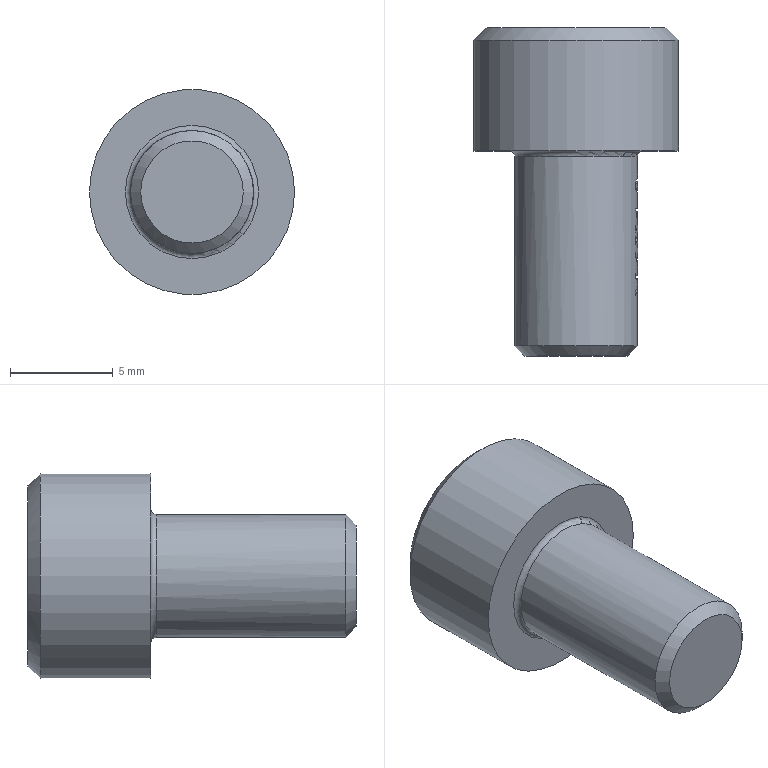Part | STEP file | solid 55 | 1 solid | 96 faces | box 10 x 16 x 10 mm | volume 680.986 mm3 | plane 53 | other 27 | cylinder 7 | sphere 6 | cone 2 | torus 1 | commonest cylinder face diameters 6 x6 10 x1